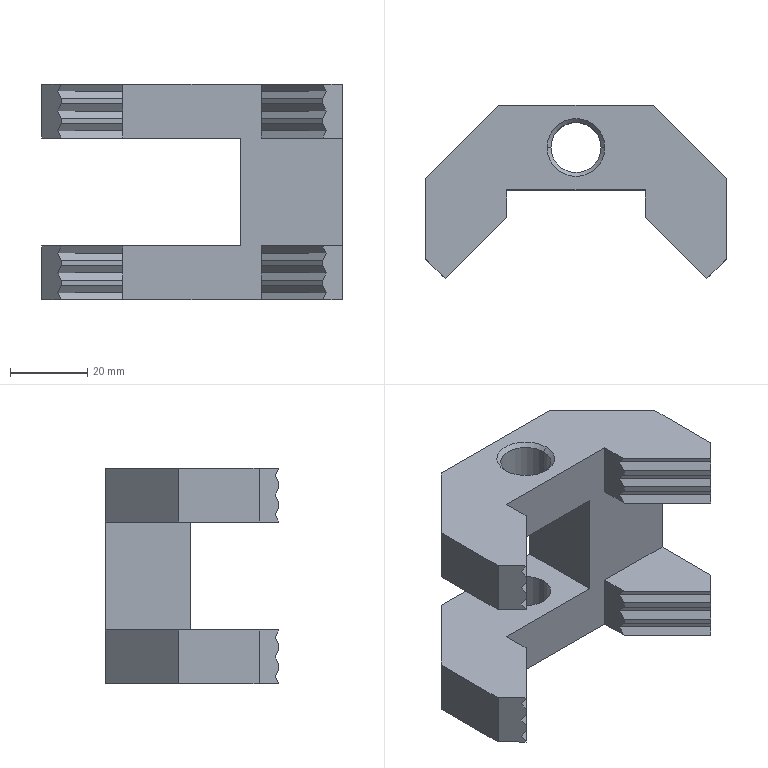Part | SolidWorks | features ICE 3, MirrorPattern 2, Chamfer 1, Extrusion 1 | 1 solid | 63 faces | box 78 x 44.997 x 56 mm | volume 64045 mm3 | plane 55 | cone 4 | cylinder 4 | commonest cylinder face diameters 13 x4